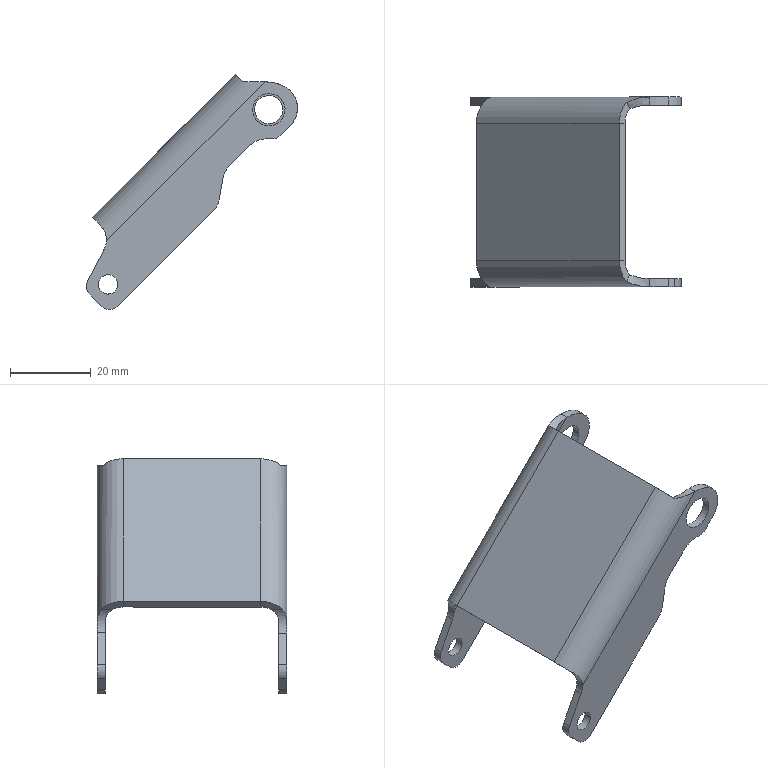Part | SolidWorks | features BaseBody 1 | 1 solid | 61 faces | box 52.277 x 47.024 x 58.146 mm | volume 8142 mm3 | cylinder 31 | plane 28 | spline 2 | commonest cylinder face diameters 10 x8 6 x6 4.8 x4 12 x3 7 x2 8 x2